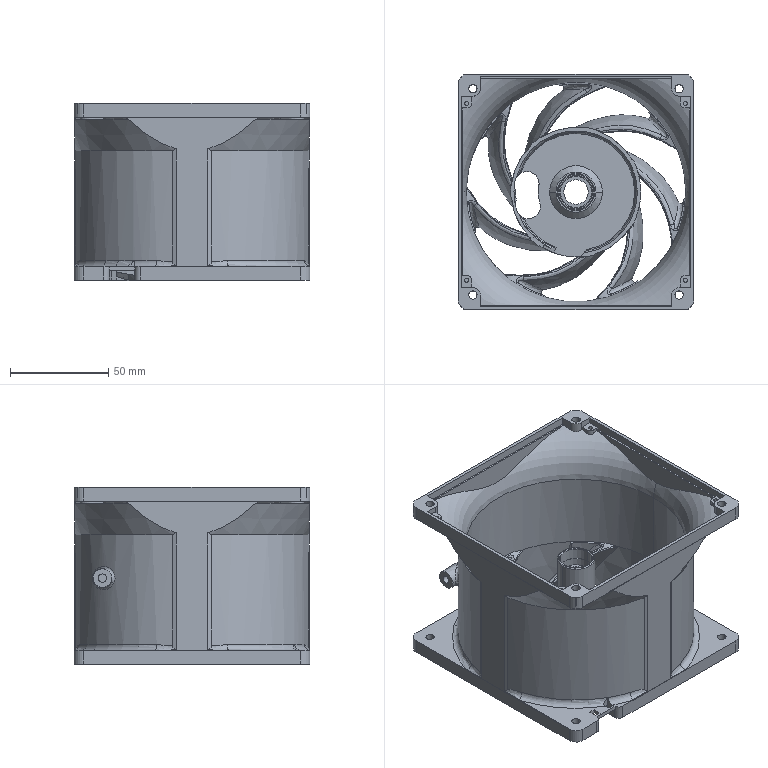NC program | NX | posted with a generic post | part box 120 x 120 x 90.2 mm
Lines 1 to 816 of 941997:
N10 G17 G21 G94 G90
(2D斜开粗_COPY , TOOL : D12-C)
N12 T02 M6
N14 G54
N16 G17 G0 G90 X-37.799 Y-23.146 S7500 M3
N18 G43 Z50.8 H2
N20 Z1.
N22 G94 G1 Y-23.017 Z0.995 F500.
N24 X-37.977 Y-22.719 Z0.983
N26 X-38.274 Y-22.542 Z0.971
N28 X-38.661 Z0.958
N30 X-38.995 Y-22.735 Z0.944
N32 X-39.188 Y-23.221 Z0.926
N34 X-38.995 Y-23.707 Z0.908
N36 X-38.641 Y-23.911 Z0.894
N38 X-38.124 Y-23.835 Z0.875
N40 X-37.799 Y-23.425 Z0.857
N42 Y-23.017 Z0.843
N44 X-37.977 Y-22.719 Z0.831
N46 X-38.274 Y-22.542 Z0.819
N48 X-38.661 Z0.805
N50 X-38.995 Y-22.735 Z0.792
N52 X-39.188 Y-23.221 Z0.773
N54 X-38.995 Y-23.707 Z0.755
N56 X-38.641 Y-23.911 Z0.741
N58 X-38.124 Y-23.835 Z0.723
N60 X-37.799 Y-23.425 Z0.704
N62 Y-23.017 Z0.69
N64 X-37.977 Y-22.719 Z0.678
N66 X-38.274 Y-22.542 Z0.666
N68 X-38.661 Z0.652
N70 X-38.995 Y-22.735 Z0.639
N72 X-39.188 Y-23.221 Z0.621
N74 X-38.995 Y-23.707 Z0.602
N76 X-38.641 Y-23.911 Z0.588
N78 X-38.124 Y-23.835 Z0.57
N80 X-37.799 Y-23.425 Z0.552
N82 Y-23.017 Z0.537
N84 X-37.977 Y-22.719 Z0.525
N86 X-38.274 Y-22.542 Z0.513
N88 X-38.661 Z0.5
N90 X-38.995 Y-22.735 Z0.486
N92 X-39.188 Y-23.221 Z0.468
N94 X-38.995 Y-23.707 Z0.45
N96 X-38.641 Y-23.911 Z0.435
N98 X-38.124 Y-23.835 Z0.417
N100 X-37.799 Y-23.425 Z0.399
N102 Y-23.017 Z0.385
N104 X-37.977 Y-22.719 Z0.372
N106 X-38.274 Y-22.542 Z0.36
N108 X-38.661 Z0.347
N110 X-38.995 Y-22.735 Z0.333
N112 X-39.188 Y-23.221 Z0.315
N114 X-38.995 Y-23.707 Z0.297
N116 X-38.641 Y-23.911 Z0.283
N118 X-38.124 Y-23.835 Z0.264
N120 X-37.799 Y-23.425 Z0.246
N122 Y-23.017 Z0.232
N124 X-37.977 Y-22.719 Z0.22
N126 X-38.274 Y-22.542 Z0.208
N128 X-38.661 Z0.194
N130 X-38.995 Y-22.735 Z0.181
N132 X-39.188 Y-23.221 Z0.162
N134 X-38.995 Y-23.707 Z0.144
N136 X-38.641 Y-23.911 Z0.13
N138 X-38.124 Y-23.835 Z0.112
N140 X-37.799 Y-23.425 Z0.093
N142 Y-23.017 Z0.079
N144 X-37.977 Y-22.719 Z0.067
N146 X-38.274 Y-22.542 Z0.055
N148 X-38.661 Z0.041
N150 X-38.995 Y-22.735 Z0.028
N152 X-39.188 Y-23.221 Z0.01
N154 X-38.995 Y-23.707 Z-0.009
N156 X-38.641 Y-23.911 Z-0.023
N158 X-38.124 Y-23.835 Z-0.041
N160 X-37.799 Y-23.425 Z-0.059
N162 Y-23.017 Z-0.074
N164 X-37.977 Y-22.719 Z-0.086
N166 X-38.274 Y-22.542 Z-0.098
N168 X-38.661 Z-0.111
N170 X-38.995 Y-22.735 Z-0.125
N172 X-39.188 Y-23.221 Z-0.143
N174 X-38.995 Y-23.707 Z-0.161
N176 X-38.641 Y-23.911 Z-0.176
N178 X-38.124 Y-23.835 Z-0.194
N180 X-37.799 Y-23.425 Z-0.212
N182 Y-23.017 Z-0.226
N184 X-37.977 Y-22.719 Z-0.239
N186 X-38.274 Y-22.542 Z-0.251
N188 X-38.661 Z-0.264
N190 X-38.995 Y-22.735 Z-0.278
N192 X-39.188 Y-23.221 Z-0.296
N194 X-38.995 Y-23.707 Z-0.314
N196 X-38.641 Y-23.911 Z-0.328
N198 X-38.124 Y-23.835 Z-0.347
N200 X-37.799 Y-23.425 Z-0.365
N202 Y-23.017 Z-0.379
N204 X-37.977 Y-22.719 Z-0.391
N206 X-38.274 Y-22.542 Z-0.403
N208 X-38.661 Z-0.417
N210 X-38.995 Y-22.735 Z-0.43
N212 X-39.188 Y-23.221 Z-0.449
N214 X-38.995 Y-23.707 Z-0.467
N216 X-38.641 Y-23.911 Z-0.481
N218 X-38.124 Y-23.835 Z-0.499
N220 X-37.799 Y-23.425 Z-0.518
N222 Y-23.017 Z-0.532
N224 X-37.977 Y-22.719 Z-0.544
N226 X-38.274 Y-22.542 Z-0.556
N228 X-38.661 Z-0.57
N230 X-38.995 Y-22.735 Z-0.583
N232 X-39.188 Y-23.221 Z-0.601
N234 X-38.995 Y-23.707 Z-0.62
N236 X-38.641 Y-23.911 Z-0.634
N238 X-38.124 Y-23.835 Z-0.652
N240 X-37.799 Y-23.425 Z-0.67
N242 Y-23.017 Z-0.685
N244 X-37.977 Y-22.719 Z-0.697
N246 X-38.274 Y-22.542 Z-0.709
N248 X-38.661 Z-0.722
N250 X-38.995 Y-22.735 Z-0.736
N252 X-39.188 Y-23.221 Z-0.754
N254 X-38.995 Y-23.707 Z-0.772
N256 X-38.641 Y-23.911 Z-0.787
N258 X-38.124 Y-23.835 Z-0.805
N260 X-37.799 Y-23.425 Z-0.823
N262 Y-23.017 Z-0.837
N264 X-37.977 Y-22.719 Z-0.85
N266 X-38.274 Y-22.542 Z-0.862
N268 X-38.661 Z-0.875
N270 X-38.995 Y-22.735 Z-0.889
N272 X-39.188 Y-23.221 Z-0.907
N274 X-38.995 Y-23.707 Z-0.925
N276 X-38.641 Y-23.911 Z-0.939
N278 X-38.124 Y-23.835 Z-0.958
N280 X-37.799 Y-23.425 Z-0.976
N282 Y-23.017 Z-0.99
N284 X-37.977 Y-22.719 Z-1.002
N286 X-38.274 Y-22.542 Z-1.014
N288 X-38.661 Z-1.028
N290 X-38.995 Y-22.735 Z-1.041
N292 X-39.188 Y-23.221 Z-1.06
N294 X-38.995 Y-23.707 Z-1.078
N296 X-38.641 Y-23.911 Z-1.092
N298 X-38.124 Y-23.835 Z-1.11
N300 X-37.799 Y-23.425 Z-1.129
N302 Y-23.017 Z-1.143
N304 X-37.977 Y-22.719 Z-1.155
N306 X-38.274 Y-22.542 Z-1.167
N308 X-38.661 Z-1.181
N310 X-38.995 Y-22.735 Z-1.194
N312 X-39.188 Y-23.221 Z-1.212
N314 X-38.995 Y-23.707 Z-1.231
N316 X-38.641 Y-23.911 Z-1.245
N318 X-38.124 Y-23.835 Z-1.263
N320 X-37.799 Y-23.425 Z-1.281
N322 Y-23.017 Z-1.296
N324 X-37.977 Y-22.719 Z-1.308
N326 X-38.274 Y-22.542 Z-1.32
N328 X-38.661 Z-1.333
N330 X-38.995 Y-22.735 Z-1.347
N332 X-39.188 Y-23.221 Z-1.365
N334 X-38.995 Y-23.707 Z-1.383
N336 X-38.641 Y-23.911 Z-1.398
N338 X-38.124 Y-23.835 Z-1.416
N340 X-37.799 Y-23.425 Z-1.434
N342 Y-23.017 Z-1.448
N344 X-37.977 Y-22.719 Z-1.461
N346 X-38.274 Y-22.542 Z-1.473
N348 X-38.661 Z-1.486
N350 X-38.995 Y-22.735 Z-1.5
N352 X-39.188 Y-23.221 Z-1.518
N354 X-38.995 Y-23.707 Z-1.536
N356 X-38.641 Y-23.911 Z-1.55
N358 X-38.124 Y-23.835 Z-1.569
N360 X-37.799 Y-23.425 Z-1.587
N362 Y-23.017 Z-1.601
N364 X-37.977 Y-22.719 Z-1.613
N366 X-38.274 Y-22.542 Z-1.625
N368 X-38.661 Z-1.639
N370 X-38.995 Y-22.735 Z-1.652
N372 X-39.188 Y-23.221 Z-1.671
N374 X-38.995 Y-23.707 Z-1.689
N376 X-38.641 Y-23.911 Z-1.703
N378 X-38.124 Y-23.835 Z-1.721
N380 X-37.799 Y-23.425 Z-1.74
N382 Y-23.017 Z-1.754
N384 X-37.977 Y-22.719 Z-1.766
N386 X-38.274 Y-22.542 Z-1.778
N388 X-38.661 Z-1.792
N390 X-38.995 Y-22.735 Z-1.805
N392 X-39.188 Y-23.221 Z-1.823
N394 X-38.995 Y-23.707 Z-1.842
N396 X-38.641 Y-23.911 Z-1.856
N398 X-38.124 Y-23.835 Z-1.874
N400 X-37.799 Y-23.425 Z-1.892
N402 Y-23.017 Z-1.907
N404 X-37.977 Y-22.719 Z-1.919
N406 X-38.274 Y-22.542 Z-1.931
N408 X-38.661 Z-1.944
N410 X-38.995 Y-22.735 Z-1.958
N412 X-39.188 Y-23.221 Z-1.976
N414 X-38.995 Y-23.707 Z-1.994
N416 X-38.641 Y-23.911 Z-2.009
N418 X-38.124 Y-23.835 Z-2.027
N420 X-37.799 Y-23.425 Z-2.045
N422 Y-23.017 Z-2.059
N424 X-37.977 Y-22.719 Z-2.072
N426 X-38.274 Y-22.542 Z-2.084
N428 X-38.661 Z-2.097
N430 X-38.995 Y-22.735 Z-2.111
N432 X-39.188 Y-23.221 Z-2.129
N434 X-38.995 Y-23.707 Z-2.147
N436 X-38.641 Y-23.911 Z-2.161
N438 X-38.124 Y-23.835 Z-2.18
N440 X-37.799 Y-23.425 Z-2.198
N442 Y-23.017 Z-2.212
N444 X-37.977 Y-22.719 Z-2.224
N446 X-38.274 Y-22.542 Z-2.236
N448 X-38.661 Z-2.25
N450 X-38.995 Y-22.735 Z-2.263
N452 X-39.188 Y-23.221 Z-2.282
N454 X-38.995 Y-23.707 Z-2.3
N456 X-38.641 Y-23.911 Z-2.314
N458 X-38.124 Y-23.835 Z-2.332
N460 X-37.799 Y-23.425 Z-2.351
N462 Y-23.017 Z-2.365
N464 X-37.977 Y-22.719 Z-2.377
N466 X-38.274 Y-22.542 Z-2.389
N468 X-38.661 Z-2.403
N470 X-38.995 Y-22.735 Z-2.416
N472 X-39.188 Y-23.221 Z-2.434
N474 X-38.995 Y-23.707 Z-2.453
N476 X-38.641 Y-23.911 Z-2.467
N478 X-38.124 Y-23.835 Z-2.485
N480 X-37.799 Y-23.425 Z-2.503
N482 Y-23.017 Z-2.518
N484 X-37.977 Y-22.719 Z-2.53
N486 X-38.274 Y-22.542 Z-2.542
N488 X-38.661 Z-2.555
N490 X-38.995 Y-22.735 Z-2.569
N492 X-39.188 Y-23.221 Z-2.587
N494 X-38.995 Y-23.707 Z-2.605
N496 X-38.641 Y-23.911 Z-2.62
N498 X-38.124 Y-23.835 Z-2.638
N500 X-37.799 Y-23.425 Z-2.656
N502 Y-23.017 Z-2.67
N504 X-37.977 Y-22.719 Z-2.683
N506 X-38.274 Y-22.542 Z-2.695
N508 X-38.661 Z-2.708
N510 X-38.995 Y-22.735 Z-2.722
N512 X-39.188 Y-23.221 Z-2.74
N514 X-38.995 Y-23.707 Z-2.758
N516 X-38.641 Y-23.911 Z-2.772
N518 X-38.124 Y-23.835 Z-2.791
N520 X-37.799 Y-23.425 Z-2.809
N522 Y-23.017 Z-2.823
N524 X-37.977 Y-22.719 Z-2.835
N526 X-38.274 Y-22.542 Z-2.847
N528 X-38.661 Z-2.861
N530 X-38.995 Y-22.735 Z-2.874
N532 X-39.188 Y-23.221 Z-2.893
N534 X-38.995 Y-23.707 Z-2.911
N536 X-38.641 Y-23.911 Z-2.925
N538 X-38.124 Y-23.835 Z-2.943
N540 X-37.799 Y-23.425 Z-2.962
N542 Y-23.017 Z-2.976
N544 X-37.977 Y-22.719 Z-2.988
N546 X-38.274 Y-22.542 Z-3.
N548 X-38.661 Z-3.014
N550 X-38.995 Y-22.735 Z-3.027
N552 X-39.188 Y-23.221 Z-3.045
N554 X-38.995 Y-23.707 Z-3.064
N556 X-38.641 Y-23.911 Z-3.078
N558 X-38.124 Y-23.835 Z-3.096
N560 X-37.799 Y-23.425 Z-3.114
N562 Y-23.017 Z-3.129
N564 X-37.977 Y-22.719 Z-3.141
N566 X-38.274 Y-22.542 Z-3.153
N568 X-38.661 Z-3.166
N570 X-38.995 Y-22.735 Z-3.18
N572 X-39.188 Y-23.221 Z-3.198
N574 X-38.995 Y-23.707 Z-3.216
N576 X-38.641 Y-23.911 Z-3.231
N578 X-38.124 Y-23.835 Z-3.249
N580 X-37.799 Y-23.425 Z-3.267
N582 Y-23.017 Z-3.281
N584 X-37.977 Y-22.719 Z-3.293
N586 X-38.274 Y-22.542 Z-3.306
N588 X-38.661 Z-3.319
N590 X-38.995 Y-22.735 Z-3.333
N592 X-39.188 Y-23.221 Z-3.351
N594 X-38.995 Y-23.707 Z-3.369
N596 X-38.641 Y-23.911 Z-3.383
N598 X-38.124 Y-23.835 Z-3.402
N600 X-37.799 Y-23.425 Z-3.42
N602 Y-23.017 Z-3.434
N604 X-37.977 Y-22.719 Z-3.446
N606 X-38.274 Y-22.542 Z-3.458
N608 X-38.661 Z-3.472
N610 X-38.995 Y-22.735 Z-3.485
N612 X-39.188 Y-23.221 Z-3.504
N614 X-38.995 Y-23.707 Z-3.522
N616 X-38.641 Y-23.911 Z-3.536
N618 X-38.124 Y-23.835 Z-3.554
N620 X-37.799 Y-23.425 Z-3.573
N622 Y-23.017 Z-3.587
N624 X-37.977 Y-22.719 Z-3.599
N626 X-38.274 Y-22.542 Z-3.611
N628 X-38.661 Z-3.625
N630 X-38.995 Y-22.735 Z-3.638
N632 X-39.188 Y-23.221 Z-3.656
N634 X-38.995 Y-23.707 Z-3.675
N636 X-38.641 Y-23.911 Z-3.689
N638 X-38.124 Y-23.835 Z-3.707
N640 X-37.799 Y-23.425 Z-3.725
N642 Y-23.017 Z-3.74
N644 X-37.977 Y-22.719 Z-3.752
N646 X-38.274 Y-22.542 Z-3.764
N648 X-38.661 Z-3.777
N650 X-38.995 Y-22.735 Z-3.791
N652 X-39.188 Y-23.221 Z-3.809
N654 X-38.995 Y-23.707 Z-3.827
N656 X-38.641 Y-23.911 Z-3.842
N658 X-38.124 Y-23.835 Z-3.86
N660 X-37.799 Y-23.425 Z-3.878
N662 Y-23.017 Z-3.892
N664 X-37.977 Y-22.719 Z-3.904
N666 X-38.274 Y-22.542 Z-3.917
N668 X-38.661 Z-3.93
N670 X-38.995 Y-22.735 Z-3.944
N672 X-39.188 Y-23.221 Z-3.962
N674 X-38.995 Y-23.707 Z-3.98
N676 X-38.641 Y-23.911 Z-3.994
N678 X-38.124 Y-23.835 Z-4.013
N680 X-37.799 Y-23.425 Z-4.031
N682 Y-23.017 Z-4.045
N684 X-37.977 Y-22.719 Z-4.057
N686 X-38.274 Y-22.542 Z-4.069
N688 X-38.661 Z-4.083
N690 X-38.995 Y-22.735 Z-4.096
N692 X-39.188 Y-23.221 Z-4.115
N694 X-38.995 Y-23.707 Z-4.133
N696 X-38.641 Y-23.911 Z-4.147
N698 X-38.124 Y-23.835 Z-4.165
N700 X-37.799 Y-23.425 Z-4.184
N702 Y-23.017 Z-4.198
N704 X-37.977 Y-22.719 Z-4.21
N706 X-38.274 Y-22.542 Z-4.222
N708 X-38.661 Z-4.236
N710 X-38.995 Y-22.735 Z-4.249
N712 X-39.188 Y-23.221 Z-4.267
N714 X-38.995 Y-23.707 Z-4.286
N716 X-38.641 Y-23.911 Z-4.3
N718 X-38.124 Y-23.835 Z-4.318
N720 X-37.799 Y-23.425 Z-4.336
N722 Y-23.017 Z-4.351
N724 X-37.977 Y-22.719 Z-4.363
N726 X-38.274 Y-22.542 Z-4.375
N728 X-38.661 Z-4.388
N730 X-38.995 Y-22.735 Z-4.402
N732 X-39.188 Y-23.221 Z-4.42
N734 X-38.995 Y-23.707 Z-4.438
N736 X-38.641 Y-23.911 Z-4.453
N738 X-38.124 Y-23.835 Z-4.471
N740 X-37.799 Y-23.425 Z-4.489
N742 Y-23.017 Z-4.503
N744 X-37.977 Y-22.719 Z-4.515
N746 X-38.274 Y-22.542 Z-4.528
N748 X-38.661 Z-4.541
N750 X-38.995 Y-22.735 Z-4.555
N752 X-39.188 Y-23.221 Z-4.573
N754 X-38.995 Y-23.707 Z-4.591
N756 X-38.641 Y-23.911 Z-4.605
N758 X-38.124 Y-23.835 Z-4.624
N760 X-37.799 Y-23.425 Z-4.642
N762 Y-23.017 Z-4.656
N764 X-37.977 Y-22.719 Z-4.668
N766 X-38.274 Y-22.542 Z-4.68
N768 X-38.661 Z-4.694
N770 X-38.995 Y-22.735 Z-4.707
N772 X-39.188 Y-23.221 Z-4.726
N774 X-38.995 Y-23.707 Z-4.744
N776 X-38.641 Y-23.911 Z-4.758
N778 X-38.124 Y-23.835 Z-4.776
N780 X-37.799 Y-23.425 Z-4.795
N782 Y-23.017 Z-4.809
N784 X-37.977 Y-22.719 Z-4.821
N786 X-38.274 Y-22.542 Z-4.833
N788 X-38.661 Z-4.847
N790 X-38.995 Y-22.735 Z-4.86
N792 X-39.188 Y-23.221 Z-4.878
N794 X-38.995 Y-23.707 Z-4.897
N796 X-38.641 Y-23.911 Z-4.911
N798 X-38.124 Y-23.835 Z-4.929
N800 X-37.799 Y-23.425 Z-4.947
N802 Y-23.017 Z-4.962
N804 X-37.977 Y-22.719 Z-4.974
N806 X-38.274 Y-22.542 Z-4.986
N808 X-38.661 Z-4.999
N810 X-38.995 Y-22.735 Z-5.013
N812 X-39.188 Y-23.221 Z-5.031
N814 X-38.995 Y-23.707 Z-5.049
N816 X-38.641 Y-23.911 Z-5.064
N818 X-38.124 Y-23.835 Z-5.082
N820 X-37.799 Y-23.425 Z-5.1
N822 Y-23.017 Z-5.114
N824 X-37.977 Y-22.719 Z-5.126
N826 X-38.274 Y-22.542 Z-5.139
N828 X-38.661 Z-5.152
N830 X-38.995 Y-22.735 Z-5.166
N832 X-39.188 Y-23.221 Z-5.184
N834 X-38.995 Y-23.707 Z-5.202
N836 X-38.641 Y-23.911 Z-5.216
N838 X-38.124 Y-23.835 Z-5.235
N840 X-37.799 Y-23.425 Z-5.253
N842 Y-23.017 Z-5.267
N844 X-37.977 Y-22.719 Z-5.279
N846 X-38.274 Y-22.542 Z-5.291
N848 X-38.661 Z-5.305
N850 X-38.995 Y-22.735 Z-5.318
N852 X-39.188 Y-23.221 Z-5.337
N854 X-38.995 Y-23.707 Z-5.355
N856 X-38.641 Y-23.911 Z-5.369
N858 X-38.124 Y-23.835 Z-5.387
N860 X-37.799 Y-23.425 Z-5.406
N862 Y-23.017 Z-5.42
N864 X-37.977 Y-22.719 Z-5.432
N866 X-38.274 Y-22.542 Z-5.444
N868 X-38.661 Z-5.458
N870 X-38.995 Y-22.735 Z-5.471
N872 X-39.188 Y-23.221 Z-5.489
N874 X-38.995 Y-23.707 Z-5.508
N876 X-38.641 Y-23.911 Z-5.522
N878 X-38.124 Y-23.835 Z-5.54
N880 X-37.799 Y-23.425 Z-5.558
N882 Y-23.017 Z-5.573
N884 X-37.977 Y-22.719 Z-5.585
N886 X-38.274 Y-22.542 Z-5.597
N888 X-38.661 Z-5.61
N890 X-38.995 Y-22.735 Z-5.624
N892 X-39.188 Y-23.221 Z-5.642
N894 X-38.995 Y-23.707 Z-5.66
N896 X-38.641 Y-23.911 Z-5.675
N898 X-38.124 Y-23.835 Z-5.693
N900 X-37.799 Y-23.425 Z-5.711
N902 Y-23.017 Z-5.725
N904 X-37.977 Y-22.719 Z-5.737
N906 X-38.274 Y-22.542 Z-5.75
N908 X-38.661 Z-5.763
N910 X-38.995 Y-22.735 Z-5.776
N912 X-39.188 Y-23.221 Z-5.795
N914 X-38.995 Y-23.707 Z-5.813
N916 X-38.641 Y-23.911 Z-5.827
N918 X-38.124 Y-23.835 Z-5.846
N920 X-37.799 Y-23.425 Z-5.864
N922 Y-23.017 Z-5.878
N924 X-37.977 Y-22.719 Z-5.89
N926 X-38.274 Y-22.542 Z-5.902
N928 X-38.661 Z-5.916
N930 X-38.995 Y-22.735 Z-5.929
N932 X-39.188 Y-23.221 Z-5.948
N934 X-38.995 Y-23.707 Z-5.966
N936 X-38.641 Y-23.911 Z-5.98
N938 X-38.124 Y-23.835 Z-5.998
N940 X-37.799 Y-23.425 Z-6.017
N942 Y-23.017 Z-6.031
N944 X-37.977 Y-22.719 Z-6.043
N946 X-38.274 Y-22.542 Z-6.055
N948 X-38.661 Z-6.068
N950 X-38.995 Y-22.735 Z-6.082
N952 X-39.188 Y-23.221 Z-6.1
N954 X-38.995 Y-23.707 Z-6.119
N956 X-38.641 Y-23.911 Z-6.133
N958 X-38.124 Y-23.835 Z-6.151
N960 X-37.799 Y-23.425 Z-6.169
N962 Y-23.017 Z-6.184
N964 X-37.977 Y-22.719 Z-6.196
N966 X-38.274 Y-22.542 Z-6.208
N968 X-38.661 Z-6.221
N970 X-38.995 Y-22.735 Z-6.235
N972 X-39.188 Y-23.221 Z-6.253
N974 X-38.995 Y-23.707 Z-6.271
N976 X-38.641 Y-23.911 Z-6.286
N978 X-38.124 Y-23.835 Z-6.304
N980 X-37.799 Y-23.425 Z-6.322
N982 Y-23.017 Z-6.336
N984 X-37.977 Y-22.719 Z-6.348
N986 X-38.274 Y-22.542 Z-6.361
N988 X-38.661 Z-6.374
N990 X-38.995 Y-22.735 Z-6.387
N992 X-39.188 Y-23.221 Z-6.406
N994 X-38.995 Y-23.707 Z-6.424
N996 X-38.641 Y-23.911 Z-6.438
N998 X-38.124 Y-23.835 Z-6.457
N1000 X-37.799 Y-23.425 Z-6.475
N1002 Y-23.017 Z-6.489
N1004 X-37.977 Y-22.719 Z-6.501
N1006 X-38.274 Y-22.542 Z-6.513
N1008 X-38.661 Z-6.527
N1010 X-38.995 Y-22.735 Z-6.54
N1012 X-39.188 Y-23.221 Z-6.558
N1014 X-38.995 Y-23.707 Z-6.577
N1016 X-38.641 Y-23.911 Z-6.591
N1018 X-38.124 Y-23.835 Z-6.609
N1020 X-37.799 Y-23.425 Z-6.628
N1022 Y-23.017 Z-6.642
N1024 X-37.977 Y-22.719 Z-6.654
N1026 X-38.274 Y-22.542 Z-6.666
N1028 X-38.661 Z-6.679
N1030 X-38.995 Y-22.735 Z-6.693
N1032 X-39.188 Y-23.221 Z-6.711
N1034 X-38.995 Y-23.707 Z-6.729
N1036 X-38.641 Y-23.911 Z-6.744
N1038 X-38.124 Y-23.835 Z-6.762
N1040 X-37.799 Y-23.425 Z-6.78
N1042 Y-23.017 Z-6.795
N1044 X-37.977 Y-22.719 Z-6.807
N1046 X-38.274 Y-22.542 Z-6.819
N1048 X-38.661 Z-6.832
N1050 X-38.995 Y-22.735 Z-6.846
N1052 X-39.188 Y-23.221 Z-6.864
N1054 X-38.995 Y-23.707 Z-6.882
N1056 X-38.641 Y-23.911 Z-6.896
N1058 X-38.124 Y-23.835 Z-6.915
N1060 X-37.799 Y-23.425 Z-6.933
N1062 Y-23.017 Z-6.947
N1064 X-37.977 Y-22.719 Z-6.959
N1066 X-38.274 Y-22.542 Z-6.971
N1068 X-38.661 Z-6.985
N1070 X-38.995 Y-22.735 Z-6.998
N1072 X-39.188 Y-23.221 Z-7.017
N1074 X-38.995 Y-23.707 Z-7.035
N1076 X-38.641 Y-23.911 Z-7.049
N1078 X-38.124 Y-23.835 Z-7.068
N1080 X-37.799 Y-23.425 Z-7.086
N1082 Y-23.017 Z-7.1
N1084 X-37.977 Y-22.719 Z-7.112
N1086 X-38.274 Y-22.542 Z-7.124
N1088 X-38.661 Z-7.138
N1090 X-38.995 Y-22.735 Z-7.151
N1092 X-39.188 Y-23.221 Z-7.169
N1094 X-38.995 Y-23.707 Z-7.188
N1096 X-38.641 Y-23.911 Z-7.202
N1098 X-38.124 Y-23.835 Z-7.22
N1100 X-37.799 Y-23.425 Z-7.239
N1102 Y-23.017 Z-7.253
N1104 X-37.977 Y-22.719 Z-7.265
N1106 X-38.274 Y-22.542 Z-7.277
N1108 X-38.661 Z-7.29
N1110 X-38.995 Y-22.735 Z-7.304
N1112 X-39.188 Y-23.221 Z-7.322
N1114 X-38.995 Y-23.707 Z-7.34
N1116 X-38.641 Y-23.911 Z-7.355
N1118 X-38.124 Y-23.835 Z-7.373
N1120 X-37.799 Y-23.425 Z-7.391
N1122 Y-23.017 Z-7.406
N1124 X-37.977 Y-22.719 Z-7.418
N1126 X-38.274 Y-22.542 Z-7.43
N1128 X-38.661 Z-7.443
N1130 X-38.995 Y-22.735 Z-7.457
N1132 X-39.188 Y-23.221 Z-7.475
N1134 X-38.995 Y-23.707 Z-7.493
N1136 X-38.641 Y-23.911 Z-7.507
N1138 X-38.124 Y-23.835 Z-7.526
N1140 X-37.799 Y-23.425 Z-7.544
N1142 Y-23.017 Z-7.558
N1144 X-37.977 Y-22.719 Z-7.57
N1146 X-38.274 Y-22.542 Z-7.582
N1148 X-38.661 Z-7.596
N1150 X-38.995 Y-22.735 Z-7.609
N1152 X-39.188 Y-23.221 Z-7.628
N1154 X-38.995 Y-23.707 Z-7.646
N1156 X-38.641 Y-23.911 Z-7.66
N1158 X-38.124 Y-23.835 Z-7.678
N1160 X-37.799 Y-23.425 Z-7.697
N1162 Y-23.017 Z-7.711
N1164 X-37.977 Y-22.719 Z-7.723
N1166 X-38.274 Y-22.542 Z-7.735
N1168 X-38.661 Z-7.749
N1170 X-38.995 Y-22.735 Z-7.762
N1172 X-39.188 Y-23.221 Z-7.78
N1174 X-38.995 Y-23.707 Z-7.799
N1176 X-38.641 Y-23.911 Z-7.813
N1178 X-38.124 Y-23.835 Z-7.831
N1180 X-37.799 Y-23.425 Z-7.85
N1182 Y-23.017 Z-7.864
N1184 X-37.977 Y-22.719 Z-7.876
N1186 X-38.274 Y-22.542 Z-7.888
N1188 X-38.661 Z-7.901
N1190 X-38.995 Y-22.735 Z-7.915
N1192 X-39.188 Y-23.221 Z-7.933
N1194 X-38.995 Y-23.707 Z-7.951
N1196 X-38.641 Y-23.911 Z-7.966
N1198 X-38.124 Y-23.835 Z-7.984
N1200 X-37.799 Y-23.425 Z-8.002
N1202 Y-23.017 Z-8.017
N1204 X-37.977 Y-22.719 Z-8.029
N1206 X-38.274 Y-22.542 Z-8.041
N1208 X-38.661 Z-8.054
N1210 X-38.995 Y-22.735 Z-8.068
N1212 X-39.188 Y-23.221 Z-8.086
N1214 X-38.995 Y-23.707 Z-8.104
N1216 X-38.641 Y-23.911 Z-8.118
N1218 X-38.124 Y-23.835 Z-8.137
N1220 X-37.799 Y-23.425 Z-8.155
N1222 Y-23.017 Z-8.169
N1224 X-37.977 Y-22.719 Z-8.181
N1226 X-38.274 Y-22.542 Z-8.193
N1228 X-38.661 Z-8.207
N1230 X-38.995 Y-22.735 Z-8.22
N1232 X-39.188 Y-23.221 Z-8.239
N1234 X-38.995 Y-23.707 Z-8.257
N1236 X-38.641 Y-23.911 Z-8.271
N1238 X-38.124 Y-23.835 Z-8.289
N1240 X-37.799 Y-23.425 Z-8.308
N1242 Y-23.017 Z-8.322
N1244 X-37.977 Y-22.719 Z-8.334
N1246 X-38.274 Y-22.542 Z-8.346
N1248 X-38.661 Z-8.36
N1250 X-38.995 Y-22.735 Z-8.373
N1252 X-39.188 Y-23.221 Z-8.391
N1254 X-38.995 Y-23.707 Z-8.41
N1256 X-38.641 Y-23.911 Z-8.424
N1258 X-38.124 Y-23.835 Z-8.442
N1260 X-37.799 Y-23.425 Z-8.46
N1262 Y-23.017 Z-8.475
N1264 X-37.977 Y-22.719 Z-8.487
N1266 X-38.274 Y-22.542 Z-8.499
N1268 X-38.661 Z-8.512
N1270 X-38.995 Y-22.735 Z-8.526
N1272 X-39.188 Y-23.221 Z-8.544
N1274 X-38.995 Y-23.707 Z-8.562
N1276 X-38.641 Y-23.911 Z-8.577
N1278 X-38.124 Y-23.835 Z-8.595
N1280 X-37.799 Y-23.425 Z-8.613
N1282 Y-23.017 Z-8.627
N1284 X-37.977 Y-22.719 Z-8.64
N1286 X-38.274 Y-22.542 Z-8.652
N1288 X-38.661 Z-8.665
N1290 X-38.995 Y-22.735 Z-8.679
N1292 X-39.188 Y-23.221 Z-8.697
N1294 X-38.995 Y-23.707 Z-8.715
N1296 X-38.641 Y-23.911 Z-8.729
N1298 X-38.124 Y-23.835 Z-8.748
N1300 X-37.799 Y-23.425 Z-8.766
N1302 Y-23.017 Z-8.78
N1304 X-37.977 Y-22.719 Z-8.792
N1306 X-38.274 Y-22.542 Z-8.804
N1308 X-38.661 Z-8.818
N1310 X-38.995 Y-22.735 Z-8.831
N1312 X-39.188 Y-23.221 Z-8.85
N1314 X-38.995 Y-23.707 Z-8.868
N1316 X-38.641 Y-23.911 Z-8.882
N1318 X-38.124 Y-23.835 Z-8.9
N1320 X-37.799 Y-23.425 Z-8.919
N1322 Y-23.017 Z-8.933
N1324 X-37.977 Y-22.719 Z-8.945
N1326 X-38.274 Y-22.542 Z-8.957
N1328 X-38.661 Z-8.971
N1330 X-38.995 Y-22.735 Z-8.984
N1332 X-39.188 Y-23.221 Z-9.002
N1334 X-38.995 Y-23.707 Z-9.021
N1336 X-38.641 Y-23.911 Z-9.035
N1338 X-38.124 Y-23.835 Z-9.053
N1340 X-37.799 Y-23.425 Z-9.071
N1342 Y-23.017 Z-9.086
N1344 X-37.977 Y-22.719 Z-9.098
N1346 X-38.274 Y-22.542 Z-9.11
N1348 X-38.661 Z-9.123
N1350 X-38.995 Y-22.735 Z-9.137
N1352 X-39.188 Y-23.221 Z-9.155
N1354 X-38.995 Y-23.707 Z-9.173
N1356 X-38.641 Y-23.911 Z-9.188
N1358 X-38.124 Y-23.835 Z-9.206
N1360 X-37.799 Y-23.425 Z-9.224
N1362 Y-23.017 Z-9.238
N1364 X-37.977 Y-22.719 Z-9.251
N1366 X-38.274 Y-22.542 Z-9.263
N1368 X-38.661 Z-9.276
N1370 X-38.995 Y-22.735 Z-9.29
N1372 X-39.188 Y-23.221 Z-9.308
N1374 X-38.995 Y-23.707 Z-9.326
N1376 X-38.641 Y-23.911 Z-9.34
N1378 X-38.124 Y-23.835 Z-9.359
N1380 X-37.799 Y-23.425 Z-9.377
N1382 Y-23.017 Z-9.391
N1384 X-37.977 Y-22.719 Z-9.403
N1386 X-38.274 Y-22.542 Z-9.415
N1388 X-38.661 Z-9.429
N1390 X-38.995 Y-22.735 Z-9.442
N1392 X-39.188 Y-23.221 Z-9.461
N1394 X-38.995 Y-23.707 Z-9.479
N1396 X-38.641 Y-23.911 Z-9.493
N1398 X-38.124 Y-23.835 Z-9.511
N1400 X-37.799 Y-23.425 Z-9.53
N1402 Y-23.017 Z-9.544
N1404 X-37.977 Y-22.719 Z-9.556
N1406 X-38.274 Y-22.542 Z-9.568
N1408 X-38.661 Z-9.582
N1410 X-38.995 Y-22.735 Z-9.595
N1412 X-39.188 Y-23.221 Z-9.613
N1414 X-38.995 Y-23.707 Z-9.632
N1416 X-38.641 Y-23.911 Z-9.646
N1418 X-38.124 Y-23.835 Z-9.664
N1420 X-37.799 Y-23.425 Z-9.682
N1422 Y-23.017 Z-9.697
N1424 X-37.977 Y-22.719 Z-9.709
N1426 X-38.274 Y-22.542 Z-9.721
N1428 X-38.661 Z-9.734
N1430 X-38.995 Y-22.735 Z-9.748
N1432 X-39.188 Y-23.221 Z-9.766
N1434 X-38.995 Y-23.707 Z-9.784
N1436 X-38.641 Y-23.911 Z-9.799
N1438 X-38.124 Y-23.835 Z-9.817
N1440 X-37.799 Y-23.425 Z-9.835
N1442 Y-23.017 Z-9.849
N1444 X-37.977 Y-22.719 Z-9.862
N1446 X-38.274 Y-22.542 Z-9.874
N1448 X-38.661 Z-9.887
N1450 X-38.995 Y-22.735 Z-9.901
N1452 X-39.188 Y-23.221 Z-9.919
N1454 X-38.995 Y-23.707 Z-9.937
N1456 X-38.641 Y-23.911 Z-9.951
N1458 X-38.124 Y-23.835 Z-9.97
N1460 X-37.799 Y-23.425 Z-9.988
N1462 Y-23.017 Z-10.002
N1464 X-37.977 Y-22.719 Z-10.014
N1466 X-38.274 Y-22.542 Z-10.026
N1468 X-38.661 Z-10.04
N1470 X-38.995 Y-22.735 Z-10.053
N1472 X-39.188 Y-23.221 Z-10.072
N1474 X-38.995 Y-23.707 Z-10.09
N1476 X-38.641 Y-23.911 Z-10.104
N1478 X-38.124 Y-23.835 Z-10.122
N1480 X-37.799 Y-23.425 Z-10.141
N1482 Y-23.017 Z-10.155
N1484 X-37.977 Y-22.719 Z-10.167
N1486 X-38.274 Y-22.542 Z-10.179
N1488 X-38.661 Z-10.193
N1490 X-38.995 Y-22.735 Z-10.206
N1492 X-39.188 Y-23.221 Z-10.224
N1494 X-38.995 Y-23.707 Z-10.243
N1496 X-38.641 Y-23.911 Z-10.257
N1498 X-38.124 Y-23.835 Z-10.275
N1500 X-37.799 Y-23.425 Z-10.293
N1502 Y-23.017 Z-10.308
N1504 X-37.977 Y-22.719 Z-10.32
N1506 X-38.274 Y-22.542 Z-10.332
N1508 X-38.661 Z-10.345
N1510 X-38.995 Y-22.735 Z-10.359
N1512 X-39.188 Y-23.221 Z-10.377
N1514 X-38.995 Y-23.707 Z-10.395
N1516 X-38.641 Y-23.911 Z-10.41
N1518 X-38.124 Y-23.835 Z-10.428
N1520 X-37.799 Y-23.425 Z-10.446
N1522 Y-23.017 Z-10.46
N1524 X-37.977 Y-22.719 Z-10.473
N1526 X-38.274 Y-22.542 Z-10.485
N1528 X-38.661 Z-10.498
N1530 X-38.995 Y-22.735 Z-10.512
N1532 X-39.188 Y-23.221 Z-10.53
N1534 X-38.995 Y-23.707 Z-10.548
N1536 X-38.641 Y-23.911 Z-10.562
N1538 X-38.124 Y-23.835 Z-10.581
N1540 X-37.799 Y-23.425 Z-10.599
N1542 Y-23.017 Z-10.613
N1544 X-37.977 Y-22.719 Z-10.625
N1546 X-38.274 Y-22.542 Z-10.637
N1548 X-38.661 Z-10.651
N1550 X-38.995 Y-22.735 Z-10.664
N1552 X-39.188 Y-23.221 Z-10.683
N1554 X-38.995 Y-23.707 Z-10.701
N1556 X-38.641 Y-23.911 Z-10.715
N1558 X-38.124 Y-23.835 Z-10.733
N1560 X-37.799 Y-23.425 Z-10.752
N1562 Y-23.017 Z-10.766
N1564 X-37.977 Y-22.719 Z-10.778
N1566 X-38.274 Y-22.542 Z-10.79
N1568 X-38.661 Z-10.804
N1570 X-38.995 Y-22.735 Z-10.817
N1572 X-39.188 Y-23.221 Z-10.835
N1574 X-38.995 Y-23.707 Z-10.854
N1576 X-38.641 Y-23.911 Z-10.868
N1578 X-38.124 Y-23.835 Z-10.886
N1580 X-37.799 Y-23.425 Z-10.904
N1582 Y-23.017 Z-10.919
N1584 X-37.977 Y-22.719 Z-10.931
N1586 X-38.274 Y-22.542 Z-10.943
N1588 X-38.478 Z-10.95
N1590 G3 X-39.158 Y-23.221 R0.679
N1592 X-38.478 Y-22.542 R-0.679
N1594 G1 Z-10.75
N1596 G0 Z50.8
(动态洗_COPY , TOOL : D12-C)
N1598 X44.233 Y-0.281
N1600 Z4.15
N1602 Z0.
N1604 G3 X44.233 Y-0.281 Z-0.462 I1.844 J3.791 F900.
N1606 X44.233 Y-0.281 Z-0.925 I1.844 J3.791
N1608 X44.233 Y-0.281 Z-1.387 I1.844 J3.791
N1610 X44.233 Y-0.281 Z-1.85 I1.844 J3.791
N1612 X44.233 Y-0.281 Z-2.312 I1.844 J3.791
N1614 X44.233 Y-0.281 Z-2.774 I1.844 J3.791
N1616 X44.233 Y-0.281 Z-3.237 I1.844 J3.791
N1618 X44.233 Y-0.281 Z-3.699 I1.844 J3.791
N1620 X44.233 Y-0.281 Z-4.162 I1.844 J3.791
N1622 X44.233 Y-0.281 Z-4.624 I1.844 J3.791
N1624 X44.233 Y-0.281 Z-5.086 I1.844 J3.791